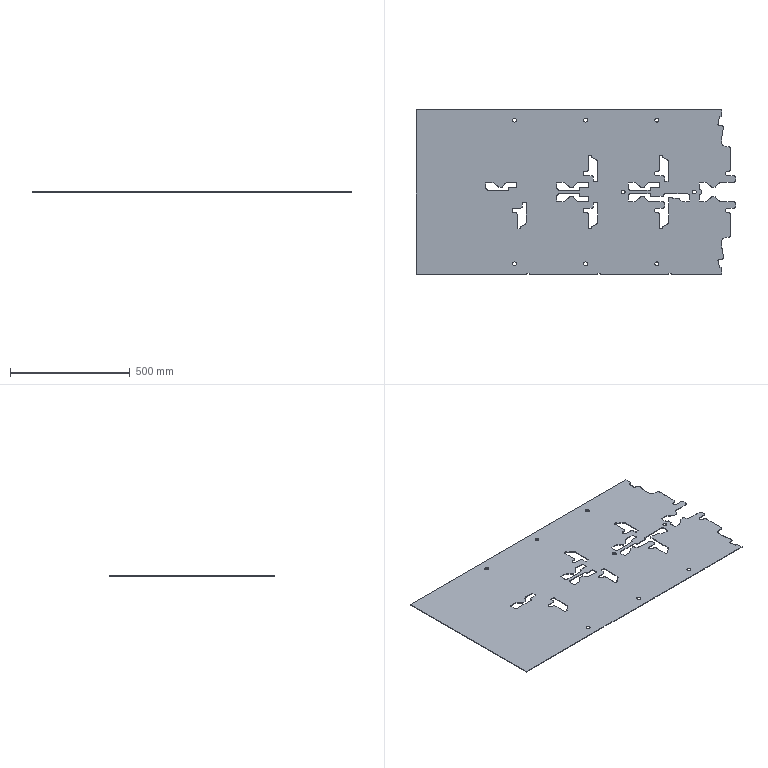Part | STEP file | lll_id350_x_t | 1 solid | 481 faces | box 1334 x 685 x 2.5 mm | volume 2100042 mm3 | cylinder 325 | plane 156 | commonest cylinder face diameters 6 x100 8 x23 20 x21 20.001 x11 16.1 x8 17.001 x8